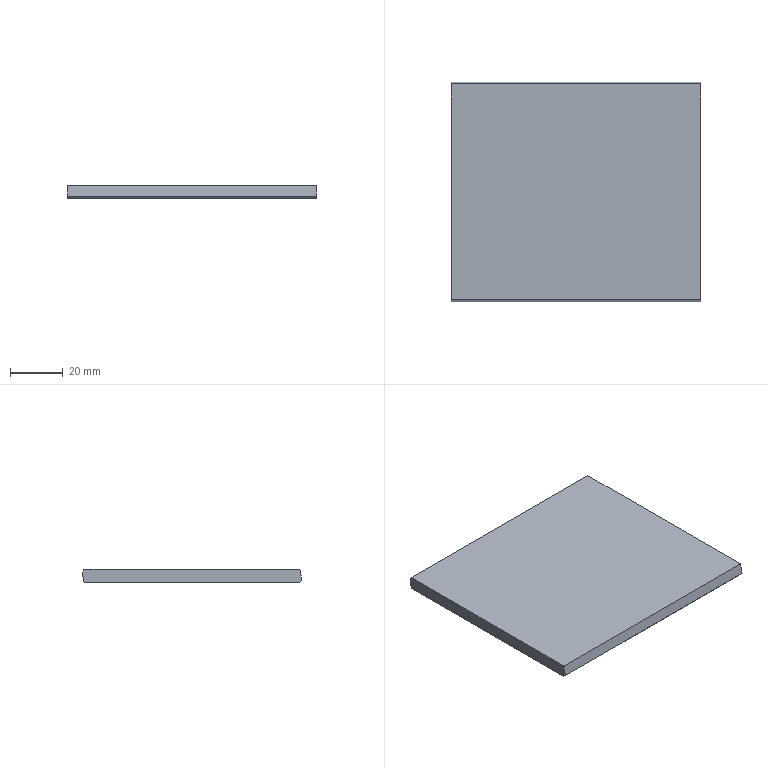Part | STEP file | Vibrator side plate_default | 1 solid | 8 faces | box 95 x 83.558 x 5 mm | volume 39344 mm3 | plane 8
STEP:
#1=CARTESIAN_POINT('',(0.,0.,0.));
#2=DIRECTION('',(0.,0.,1.));
#3=DIRECTION('',(1.,0.,0.));
#4=AXIS2_PLACEMENT_3D('',#1,#2,#3);
#5=CARTESIAN_POINT('',(-47.5,41.5,0.));
#6=VERTEX_POINT('',#5);
#7=CARTESIAN_POINT('',(-47.5,-40.5,0.));
#8=VERTEX_POINT('',#7);
#9=CARTESIAN_POINT('',(-47.5,-41.5,0.));
#10=DIRECTION('',(0.,-1.,0.));
#11=VECTOR('',#10,1.);
#12=LINE('',#9,#11);
#13=CARTESIAN_POINT('',(-47.5,-40.618,5.));
#14=DIRECTION('',(1.,0.,0.));
#15=DIRECTION('',(0.,0.,-1.));
#16=AXIS2_PLACEMENT_3D('',#13,#14,#15);
#17=PLANE('',#16);
#18=CARTESIAN_POINT('',(5.,-0.8816));
#19=DIRECTION('',(0.,-1.));
#20=VECTOR('',#19,1.);
#21=LINE('',#18,#20);
#22=(GEOMETRIC_REPRESENTATION_CONTEXT(2)PARAMETRIC_REPRESENTATION_CONTEXT()REPRESENTATION_CONTEXT('',''));
#23=DEFINITIONAL_REPRESENTATION('',(#21),#22);
#24=PCURVE('',#17,#23);
#25=CARTESIAN_POINT('',(0.,0.,0.));
#26=DIRECTION('',(0.,0.,1.));
#27=DIRECTION('',(1.,0.,0.));
#28=AXIS2_PLACEMENT_3D('',#25,#26,#27);
#29=PLANE('',#28);
#30=CARTESIAN_POINT('',(-47.5,-41.5));
#31=DIRECTION('',(0.,-1.));
#32=VECTOR('',#31,1.);
#33=LINE('',#30,#32);
#34=(GEOMETRIC_REPRESENTATION_CONTEXT(2)PARAMETRIC_REPRESENTATION_CONTEXT()REPRESENTATION_CONTEXT('',''));
#35=DEFINITIONAL_REPRESENTATION('',(#33),#34);
#36=PCURVE('',#29,#35);
#37=SURFACE_CURVE('',#12,(#24,#36),.PCURVE_S1.);
#38=EDGE_CURVE('',#6,#8,#37,.T.);
#39=ORIENTED_EDGE('',*,*,#38,.T.);
#40=CARTESIAN_POINT('',(-47.5,-41.35,0.8501));
#41=VERTEX_POINT('',#40);
#42=CARTESIAN_POINT('',(-47.5,-41.35,0.8501));
#43=DIRECTION('',(0.,-0.7071,0.7071));
#44=VECTOR('',#43,1.);
#45=LINE('',#42,#44);
#46=CARTESIAN_POINT('',(4.15,-0.7317));
#47=DIRECTION('',(-0.7071,-0.7071));
#48=VECTOR('',#47,1.);
#49=LINE('',#46,#48);
#50=(GEOMETRIC_REPRESENTATION_CONTEXT(2)PARAMETRIC_REPRESENTATION_CONTEXT()REPRESENTATION_CONTEXT('',''));
#51=DEFINITIONAL_REPRESENTATION('',(#49),#50);
#52=PCURVE('',#17,#51);
#53=CARTESIAN_POINT('',(47.5,-41.35,0.8501));
#54=DIRECTION('',(0.,0.7071,0.7071));
#55=DIRECTION('',(1.,0.,0.));
#56=AXIS2_PLACEMENT_3D('',#53,#54,#55);
#57=PLANE('',#56);
#58=CARTESIAN_POINT('',(-95.,0.));
#59=DIRECTION('',(0.,-1.));
#60=VECTOR('',#59,1.);
#61=LINE('',#58,#60);
#62=(GEOMETRIC_REPRESENTATION_CONTEXT(2)PARAMETRIC_REPRESENTATION_CONTEXT()REPRESENTATION_CONTEXT('',''));
#63=DEFINITIONAL_REPRESENTATION('',(#61),#62);
#64=PCURVE('',#57,#63);
#65=SURFACE_CURVE('',#45,(#52,#64),.PCURVE_S1.);
#66=EDGE_CURVE('',#8,#41,#65,.T.);
#67=ORIENTED_EDGE('',*,*,#66,.T.);
#68=CARTESIAN_POINT('',(-47.5,-40.618,5.));
#69=VERTEX_POINT('',#68);
#70=CARTESIAN_POINT('',(-47.5,-40.618,5.));
#71=DIRECTION('',(0.,-0.1736,-0.9848));
#72=VECTOR('',#71,1.);
#73=LINE('',#70,#72);
#74=CARTESIAN_POINT('',(0.,0.));
#75=DIRECTION('',(0.9848,-0.1736));
#76=VECTOR('',#75,1.);
#77=LINE('',#74,#76);
#78=(GEOMETRIC_REPRESENTATION_CONTEXT(2)PARAMETRIC_REPRESENTATION_CONTEXT()REPRESENTATION_CONTEXT('',''));
#79=DEFINITIONAL_REPRESENTATION('',(#77),#78);
#80=PCURVE('',#17,#79);
#81=CARTESIAN_POINT('',(47.5,-40.618,5.));
#82=DIRECTION('',(0.,0.9848,-0.1736));
#83=DIRECTION('',(0.,0.1736,0.9848));
#84=AXIS2_PLACEMENT_3D('',#81,#82,#83);
#85=PLANE('',#84);
#86=CARTESIAN_POINT('',(0.,-95.));
#87=DIRECTION('',(-1.,0.));
#88=VECTOR('',#87,1.);
#89=LINE('',#86,#88);
#90=(GEOMETRIC_REPRESENTATION_CONTEXT(2)PARAMETRIC_REPRESENTATION_CONTEXT()REPRESENTATION_CONTEXT('',''));
#91=DEFINITIONAL_REPRESENTATION('',(#89),#90);
#92=PCURVE('',#85,#91);
#93=SURFACE_CURVE('',#73,(#80,#92),.PCURVE_S1.);
#94=EDGE_CURVE('',#69,#41,#93,.T.);
#95=ORIENTED_EDGE('',*,*,#94,.F.);
#96=CARTESIAN_POINT('',(-47.5,41.518,5.));
#97=VERTEX_POINT('',#96);
#98=CARTESIAN_POINT('',(-47.5,-40.618,5.));
#99=DIRECTION('',(0.,-1.,0.));
#100=VECTOR('',#99,1.);
#101=LINE('',#98,#100);
#102=CARTESIAN_POINT('',(0.,0.));
#103=DIRECTION('',(0.,-1.));
#104=VECTOR('',#103,1.);
#105=LINE('',#102,#104);
#106=(GEOMETRIC_REPRESENTATION_CONTEXT(2)PARAMETRIC_REPRESENTATION_CONTEXT()REPRESENTATION_CONTEXT('',''));
#107=DEFINITIONAL_REPRESENTATION('',(#105),#106);
#108=PCURVE('',#17,#107);
#109=CARTESIAN_POINT('',(0.,0.8816,5.));
#110=DIRECTION('',(0.,0.,1.));
#111=DIRECTION('',(1.,0.,0.));
#112=AXIS2_PLACEMENT_3D('',#109,#110,#111);
#113=PLANE('',#112);
#114=CARTESIAN_POINT('',(-47.5,-41.5));
#115=DIRECTION('',(0.,-1.));
#116=VECTOR('',#115,1.);
#117=LINE('',#114,#116);
#118=(GEOMETRIC_REPRESENTATION_CONTEXT(2)PARAMETRIC_REPRESENTATION_CONTEXT()REPRESENTATION_CONTEXT('',''));
#119=DEFINITIONAL_REPRESENTATION('',(#117),#118);
#120=PCURVE('',#113,#119);
#121=SURFACE_CURVE('',#101,(#108,#120),.PCURVE_S1.);
#122=EDGE_CURVE('',#97,#69,#121,.T.);
#123=ORIENTED_EDGE('',*,*,#122,.F.);
#124=CARTESIAN_POINT('',(-47.5,42.208,4.015));
#125=VERTEX_POINT('',#124);
#126=CARTESIAN_POINT('',(-47.5,41.518,5.));
#127=DIRECTION('',(0.,0.5736,-0.8192));
#128=VECTOR('',#127,1.);
#129=LINE('',#126,#128);
#130=CARTESIAN_POINT('',(0.,82.137));
#131=DIRECTION('',(0.8192,0.5736));
#132=VECTOR('',#131,1.);
#133=LINE('',#130,#132);
#134=(GEOMETRIC_REPRESENTATION_CONTEXT(2)PARAMETRIC_REPRESENTATION_CONTEXT()REPRESENTATION_CONTEXT('',''));
#135=DEFINITIONAL_REPRESENTATION('',(#133),#134);
#136=PCURVE('',#17,#135);
#137=CARTESIAN_POINT('',(0.,41.518,5.));
#138=DIRECTION('',(0.,0.8192,0.5736));
#139=DIRECTION('',(1.,0.,0.));
#140=AXIS2_PLACEMENT_3D('',#137,#138,#139);
#141=PLANE('',#140);
#142=CARTESIAN_POINT('',(-47.5,0.));
#143=DIRECTION('',(0.,1.));
#144=VECTOR('',#143,1.);
#145=LINE('',#142,#144);
#146=(GEOMETRIC_REPRESENTATION_CONTEXT(2)PARAMETRIC_REPRESENTATION_CONTEXT()REPRESENTATION_CONTEXT('',''));
#147=DEFINITIONAL_REPRESENTATION('',(#145),#146);
#148=PCURVE('',#141,#147);
#149=SURFACE_CURVE('',#129,(#136,#148),.PCURVE_S1.);
#150=EDGE_CURVE('',#97,#125,#149,.T.);
#151=ORIENTED_EDGE('',*,*,#150,.T.);
#152=CARTESIAN_POINT('',(-47.5,42.382,5.));
#153=DIRECTION('',(0.,-0.1736,-0.9848));
#154=VECTOR('',#153,1.);
#155=LINE('',#152,#154);
#156=CARTESIAN_POINT('',(0.,83.));
#157=DIRECTION('',(0.9848,-0.1736));
#158=VECTOR('',#157,1.);
#159=LINE('',#156,#158);
#160=(GEOMETRIC_REPRESENTATION_CONTEXT(2)PARAMETRIC_REPRESENTATION_CONTEXT()REPRESENTATION_CONTEXT('',''));
#161=DEFINITIONAL_REPRESENTATION('',(#159),#160);
#162=PCURVE('',#17,#161);
#163=CARTESIAN_POINT('',(47.5,42.382,5.));
#164=DIRECTION('',(0.,-0.9848,0.1736));
#165=DIRECTION('',(0.,-0.1736,-0.9848));
#166=AXIS2_PLACEMENT_3D('',#163,#164,#165);
#167=PLANE('',#166);
#168=CARTESIAN_POINT('',(0.,-95.));
#169=DIRECTION('',(1.,0.));
#170=VECTOR('',#169,1.);
#171=LINE('',#168,#170);
#172=(GEOMETRIC_REPRESENTATION_CONTEXT(2)PARAMETRIC_REPRESENTATION_CONTEXT()REPRESENTATION_CONTEXT('',''));
#173=DEFINITIONAL_REPRESENTATION('',(#171),#172);
#174=PCURVE('',#167,#173);
#175=SURFACE_CURVE('',#155,(#162,#174),.PCURVE_S1.);
#176=EDGE_CURVE('',#125,#6,#175,.T.);
#177=ORIENTED_EDGE('',*,*,#176,.T.);
#178=EDGE_LOOP('',(#39,#67,#95,#123,#151,#177));
#179=FACE_BOUND('',#178,.T.);
#180=ADVANCED_FACE('',(#179),#17,.F.);
#181=ORIENTED_EDGE('',*,*,#94,.T.);
#182=CARTESIAN_POINT('',(47.5,-41.35,0.8501));
#183=VERTEX_POINT('',#182);
#184=CARTESIAN_POINT('',(47.5,-41.35,0.8501));
#185=DIRECTION('',(1.,0.,0.));
#186=VECTOR('',#185,1.);
#187=LINE('',#184,#186);
#188=CARTESIAN_POINT('',(-4.214,0.));
#189=DIRECTION('',(0.,1.));
#190=VECTOR('',#189,1.);
#191=LINE('',#188,#190);
#192=(GEOMETRIC_REPRESENTATION_CONTEXT(2)PARAMETRIC_REPRESENTATION_CONTEXT()REPRESENTATION_CONTEXT('',''));
#193=DEFINITIONAL_REPRESENTATION('',(#191),#192);
#194=PCURVE('',#85,#193);
#195=CARTESIAN_POINT('',(0.,0.));
#196=DIRECTION('',(1.,0.));
#197=VECTOR('',#196,1.);
#198=LINE('',#195,#197);
#199=(GEOMETRIC_REPRESENTATION_CONTEXT(2)PARAMETRIC_REPRESENTATION_CONTEXT()REPRESENTATION_CONTEXT('',''));
#200=DEFINITIONAL_REPRESENTATION('',(#198),#199);
#201=PCURVE('',#57,#200);
#202=SURFACE_CURVE('',#187,(#194,#201),.PCURVE_S1.);
#203=EDGE_CURVE('',#41,#183,#202,.T.);
#204=ORIENTED_EDGE('',*,*,#203,.T.);
#205=CARTESIAN_POINT('',(47.5,-40.618,5.));
#206=VERTEX_POINT('',#205);
#207=CARTESIAN_POINT('',(47.5,-40.618,5.));
#208=DIRECTION('',(0.,-0.1736,-0.9848));
#209=VECTOR('',#208,1.);
#210=LINE('',#207,#209);
#211=CARTESIAN_POINT('',(0.,0.));
#212=DIRECTION('',(-1.,0.));
#213=VECTOR('',#212,1.);
#214=LINE('',#211,#213);
#215=(GEOMETRIC_REPRESENTATION_CONTEXT(2)PARAMETRIC_REPRESENTATION_CONTEXT()REPRESENTATION_CONTEXT('',''));
#216=DEFINITIONAL_REPRESENTATION('',(#214),#215);
#217=PCURVE('',#85,#216);
#218=CARTESIAN_POINT('',(47.5,-40.618,5.));
#219=DIRECTION('',(-1.,0.,0.));
#220=DIRECTION('',(0.,0.,1.));
#221=AXIS2_PLACEMENT_3D('',#218,#219,#220);
#222=PLANE('',#221);
#223=CARTESIAN_POINT('',(0.,0.));
#224=DIRECTION('',(-0.9848,-0.1736));
#225=VECTOR('',#224,1.);
#226=LINE('',#223,#225);
#227=(GEOMETRIC_REPRESENTATION_CONTEXT(2)PARAMETRIC_REPRESENTATION_CONTEXT()REPRESENTATION_CONTEXT('',''));
#228=DEFINITIONAL_REPRESENTATION('',(#226),#227);
#229=PCURVE('',#222,#228);
#230=SURFACE_CURVE('',#210,(#217,#229),.PCURVE_S1.);
#231=EDGE_CURVE('',#206,#183,#230,.T.);
#232=ORIENTED_EDGE('',*,*,#231,.F.);
#233=CARTESIAN_POINT('',(47.5,-40.618,5.));
#234=DIRECTION('',(1.,0.,0.));
#235=VECTOR('',#234,1.);
#236=LINE('',#233,#235);
#237=CARTESIAN_POINT('',(0.,0.));
#238=DIRECTION('',(0.,1.));
#239=VECTOR('',#238,1.);
#240=LINE('',#237,#239);
#241=(GEOMETRIC_REPRESENTATION_CONTEXT(2)PARAMETRIC_REPRESENTATION_CONTEXT()REPRESENTATION_CONTEXT('',''));
#242=DEFINITIONAL_REPRESENTATION('',(#240),#241);
#243=PCURVE('',#85,#242);
#244=CARTESIAN_POINT('',(47.5,-41.5));
#245=DIRECTION('',(1.,0.));
#246=VECTOR('',#245,1.);
#247=LINE('',#244,#246);
#248=(GEOMETRIC_REPRESENTATION_CONTEXT(2)PARAMETRIC_REPRESENTATION_CONTEXT()REPRESENTATION_CONTEXT('',''));
#249=DEFINITIONAL_REPRESENTATION('',(#247),#248);
#250=PCURVE('',#113,#249);
#251=SURFACE_CURVE('',#236,(#243,#250),.PCURVE_S1.);
#252=EDGE_CURVE('',#69,#206,#251,.T.);
#253=ORIENTED_EDGE('',*,*,#252,.F.);
#254=EDGE_LOOP('',(#181,#204,#232,#253));
#255=FACE_BOUND('',#254,.T.);
#256=ADVANCED_FACE('',(#255),#85,.F.);
#257=ORIENTED_EDGE('',*,*,#231,.T.);
#258=CARTESIAN_POINT('',(47.5,-40.5,0.));
#259=VERTEX_POINT('',#258);
#260=CARTESIAN_POINT('',(47.5,-41.35,0.8501));
#261=DIRECTION('',(0.,0.7071,-0.7071));
#262=VECTOR('',#261,1.);
#263=LINE('',#260,#262);
#264=CARTESIAN_POINT('',(-4.15,-0.7317));
#265=DIRECTION('',(-0.7071,0.7071));
#266=VECTOR('',#265,1.);
#267=LINE('',#264,#266);
#268=(GEOMETRIC_REPRESENTATION_CONTEXT(2)PARAMETRIC_REPRESENTATION_CONTEXT()REPRESENTATION_CONTEXT('',''));
#269=DEFINITIONAL_REPRESENTATION('',(#267),#268);
#270=PCURVE('',#222,#269);
#271=CARTESIAN_POINT('',(0.,0.));
#272=DIRECTION('',(0.,1.));
#273=VECTOR('',#272,1.);
#274=LINE('',#271,#273);
#275=(GEOMETRIC_REPRESENTATION_CONTEXT(2)PARAMETRIC_REPRESENTATION_CONTEXT()REPRESENTATION_CONTEXT('',''));
#276=DEFINITIONAL_REPRESENTATION('',(#274),#275);
#277=PCURVE('',#57,#276);
#278=SURFACE_CURVE('',#263,(#270,#277),.PCURVE_S1.);
#279=EDGE_CURVE('',#183,#259,#278,.T.);
#280=ORIENTED_EDGE('',*,*,#279,.T.);
#281=CARTESIAN_POINT('',(47.5,41.5,0.));
#282=VERTEX_POINT('',#281);
#283=CARTESIAN_POINT('',(47.5,-41.5,0.));
#284=DIRECTION('',(0.,1.,0.));
#285=VECTOR('',#284,1.);
#286=LINE('',#283,#285);
#287=CARTESIAN_POINT('',(-5.,-0.8816));
#288=DIRECTION('',(0.,1.));
#289=VECTOR('',#288,1.);
#290=LINE('',#287,#289);
#291=(GEOMETRIC_REPRESENTATION_CONTEXT(2)PARAMETRIC_REPRESENTATION_CONTEXT()REPRESENTATION_CONTEXT('',''));
#292=DEFINITIONAL_REPRESENTATION('',(#290),#291);
#293=PCURVE('',#222,#292);
#294=CARTESIAN_POINT('',(47.5,-41.5));
#295=DIRECTION('',(0.,1.));
#296=VECTOR('',#295,1.);
#297=LINE('',#294,#296);
#298=(GEOMETRIC_REPRESENTATION_CONTEXT(2)PARAMETRIC_REPRESENTATION_CONTEXT()REPRESENTATION_CONTEXT('',''));
#299=DEFINITIONAL_REPRESENTATION('',(#297),#298);
#300=PCURVE('',#29,#299);
#301=SURFACE_CURVE('',#286,(#293,#300),.PCURVE_S1.);
#302=EDGE_CURVE('',#259,#282,#301,.T.);
#303=ORIENTED_EDGE('',*,*,#302,.T.);
#304=CARTESIAN_POINT('',(47.5,42.208,4.015));
#305=VERTEX_POINT('',#304);
#306=CARTESIAN_POINT('',(47.5,42.382,5.));
#307=DIRECTION('',(0.,-0.1736,-0.9848));
#308=VECTOR('',#307,1.);
#309=LINE('',#306,#308);
#310=CARTESIAN_POINT('',(0.,83.));
#311=DIRECTION('',(-0.9848,-0.1736));
#312=VECTOR('',#311,1.);
#313=LINE('',#310,#312);
#314=(GEOMETRIC_REPRESENTATION_CONTEXT(2)PARAMETRIC_REPRESENTATION_CONTEXT()REPRESENTATION_CONTEXT('',''));
#315=DEFINITIONAL_REPRESENTATION('',(#313),#314);
#316=PCURVE('',#222,#315);
#317=CARTESIAN_POINT('',(0.,0.));
#318=DIRECTION('',(1.,0.));
#319=VECTOR('',#318,1.);
#320=LINE('',#317,#319);
#321=(GEOMETRIC_REPRESENTATION_CONTEXT(2)PARAMETRIC_REPRESENTATION_CONTEXT()REPRESENTATION_CONTEXT('',''));
#322=DEFINITIONAL_REPRESENTATION('',(#320),#321);
#323=PCURVE('',#167,#322);
#324=SURFACE_CURVE('',#309,(#316,#323),.PCURVE_S1.);
#325=EDGE_CURVE('',#305,#282,#324,.T.);
#326=ORIENTED_EDGE('',*,*,#325,.F.);
#327=CARTESIAN_POINT('',(47.5,41.518,5.));
#328=VERTEX_POINT('',#327);
#329=CARTESIAN_POINT('',(47.5,41.518,5.));
#330=DIRECTION('',(0.,-0.5736,0.8192));
#331=VECTOR('',#330,1.);
#332=LINE('',#329,#331);
#333=CARTESIAN_POINT('',(0.,82.137));
#334=DIRECTION('',(0.8192,-0.5736));
#335=VECTOR('',#334,1.);
#336=LINE('',#333,#335);
#337=(GEOMETRIC_REPRESENTATION_CONTEXT(2)PARAMETRIC_REPRESENTATION_CONTEXT()REPRESENTATION_CONTEXT('',''));
#338=DEFINITIONAL_REPRESENTATION('',(#336),#337);
#339=PCURVE('',#222,#338);
#340=CARTESIAN_POINT('',(47.5,0.));
#341=DIRECTION('',(0.,-1.));
#342=VECTOR('',#341,1.);
#343=LINE('',#340,#342);
#344=(GEOMETRIC_REPRESENTATION_CONTEXT(2)PARAMETRIC_REPRESENTATION_CONTEXT()REPRESENTATION_CONTEXT('',''));
#345=DEFINITIONAL_REPRESENTATION('',(#343),#344);
#346=PCURVE('',#141,#345);
#347=SURFACE_CURVE('',#332,(#339,#346),.PCURVE_S1.);
#348=EDGE_CURVE('',#305,#328,#347,.T.);
#349=ORIENTED_EDGE('',*,*,#348,.T.);
#350=CARTESIAN_POINT('',(47.5,-40.618,5.));
#351=DIRECTION('',(0.,1.,0.));
#352=VECTOR('',#351,1.);
#353=LINE('',#350,#352);
#354=CARTESIAN_POINT('',(0.,0.));
#355=DIRECTION('',(0.,1.));
#356=VECTOR('',#355,1.);
#357=LINE('',#354,#356);
#358=(GEOMETRIC_REPRESENTATION_CONTEXT(2)PARAMETRIC_REPRESENTATION_CONTEXT()REPRESENTATION_CONTEXT('',''));
#359=DEFINITIONAL_REPRESENTATION('',(#357),#358);
#360=PCURVE('',#222,#359);
#361=CARTESIAN_POINT('',(47.5,-41.5));
#362=DIRECTION('',(0.,1.));
#363=VECTOR('',#362,1.);
#364=LINE('',#361,#363);
#365=(GEOMETRIC_REPRESENTATION_CONTEXT(2)PARAMETRIC_REPRESENTATION_CONTEXT()REPRESENTATION_CONTEXT('',''));
#366=DEFINITIONAL_REPRESENTATION('',(#364),#365);
#367=PCURVE('',#113,#366);
#368=SURFACE_CURVE('',#353,(#360,#367),.PCURVE_S1.);
#369=EDGE_CURVE('',#206,#328,#368,.T.);
#370=ORIENTED_EDGE('',*,*,#369,.F.);
#371=EDGE_LOOP('',(#257,#280,#303,#326,#349,#370));
#372=FACE_BOUND('',#371,.T.);
#373=ADVANCED_FACE('',(#372),#222,.F.);
#374=ORIENTED_EDGE('',*,*,#176,.F.);
#375=CARTESIAN_POINT('',(47.5,42.208,4.015));
#376=DIRECTION('',(1.,0.,0.));
#377=VECTOR('',#376,1.);
#378=LINE('',#375,#377);
#379=CARTESIAN_POINT('',(1.,0.));
#380=DIRECTION('',(0.,1.));
#381=VECTOR('',#380,1.);
#382=LINE('',#379,#381);
#383=(GEOMETRIC_REPRESENTATION_CONTEXT(2)PARAMETRIC_REPRESENTATION_CONTEXT()REPRESENTATION_CONTEXT('',''));
#384=DEFINITIONAL_REPRESENTATION('',(#382),#383);
#385=PCURVE('',#167,#384);
#386=CARTESIAN_POINT('',(47.5,1.202));
#387=DIRECTION('',(1.,0.));
#388=VECTOR('',#387,1.);
#389=LINE('',#386,#388);
#390=(GEOMETRIC_REPRESENTATION_CONTEXT(2)PARAMETRIC_REPRESENTATION_CONTEXT()REPRESENTATION_CONTEXT('',''));
#391=DEFINITIONAL_REPRESENTATION('',(#389),#390);
#392=PCURVE('',#141,#391);
#393=SURFACE_CURVE('',#378,(#385,#392),.PCURVE_S1.);
#394=EDGE_CURVE('',#125,#305,#393,.T.);
#395=ORIENTED_EDGE('',*,*,#394,.T.);
#396=ORIENTED_EDGE('',*,*,#325,.T.);
#397=CARTESIAN_POINT('',(47.5,41.5,0.));
#398=DIRECTION('',(-1.,0.,0.));
#399=VECTOR('',#398,1.);
#400=LINE('',#397,#399);
#401=CARTESIAN_POINT('',(5.077,0.));
#402=DIRECTION('',(0.,-1.));
#403=VECTOR('',#402,1.);
#404=LINE('',#401,#403);
#405=(GEOMETRIC_REPRESENTATION_CONTEXT(2)PARAMETRIC_REPRESENTATION_CONTEXT()REPRESENTATION_CONTEXT('',''));
#406=DEFINITIONAL_REPRESENTATION('',(#404),#405);
#407=PCURVE('',#167,#406);
#408=CARTESIAN_POINT('',(47.5,41.5));
#409=DIRECTION('',(-1.,0.));
#410=VECTOR('',#409,1.);
#411=LINE('',#408,#410);
#412=(GEOMETRIC_REPRESENTATION_CONTEXT(2)PARAMETRIC_REPRESENTATION_CONTEXT()REPRESENTATION_CONTEXT('',''));
#413=DEFINITIONAL_REPRESENTATION('',(#411),#412);
#414=PCURVE('',#29,#413);
#415=SURFACE_CURVE('',#400,(#407,#414),.PCURVE_S1.);
#416=EDGE_CURVE('',#282,#6,#415,.T.);
#417=ORIENTED_EDGE('',*,*,#416,.T.);
#418=EDGE_LOOP('',(#374,#395,#396,#417));
#419=FACE_BOUND('',#418,.T.);
#420=ADVANCED_FACE('',(#419),#167,.F.);
#421=ORIENTED_EDGE('',*,*,#369,.T.);
#422=CARTESIAN_POINT('',(-47.5,41.518,5.));
#423=DIRECTION('',(-1.,0.,0.));
#424=VECTOR('',#423,1.);
#425=LINE('',#422,#424);
#426=CARTESIAN_POINT('',(-47.5,40.637));
#427=DIRECTION('',(-1.,0.));
#428=VECTOR('',#427,1.);
#429=LINE('',#426,#428);
#430=(GEOMETRIC_REPRESENTATION_CONTEXT(2)PARAMETRIC_REPRESENTATION_CONTEXT()REPRESENTATION_CONTEXT('',''));
#431=DEFINITIONAL_REPRESENTATION('',(#429),#430);
#432=PCURVE('',#113,#431);
#433=CARTESIAN_POINT('',(-47.5,0.));
#434=DIRECTION('',(-1.,0.));
#435=VECTOR('',#434,1.);
#436=LINE('',#433,#435);
#437=(GEOMETRIC_REPRESENTATION_CONTEXT(2)PARAMETRIC_REPRESENTATION_CONTEXT()REPRESENTATION_CONTEXT('',''));
#438=DEFINITIONAL_REPRESENTATION('',(#436),#437);
#439=PCURVE('',#141,#438);
#440=SURFACE_CURVE('',#425,(#432,#439),.PCURVE_S1.);
#441=EDGE_CURVE('',#328,#97,#440,.T.);
#442=ORIENTED_EDGE('',*,*,#441,.T.);
#443=ORIENTED_EDGE('',*,*,#122,.T.);
#444=ORIENTED_EDGE('',*,*,#252,.T.);
#445=EDGE_LOOP('',(#421,#442,#443,#444));
#446=FACE_BOUND('',#445,.T.);
#447=ADVANCED_FACE('',(#446),#113,.T.);
#448=ORIENTED_EDGE('',*,*,#302,.F.);
#449=CARTESIAN_POINT('',(0.,-40.5,0.));
#450=DIRECTION('',(-1.,0.,0.));
#451=VECTOR('',#450,1.);
#452=LINE('',#449,#451);
#453=CARTESIAN_POINT('',(0.,-40.5));
#454=DIRECTION('',(-1.,0.));
#455=VECTOR('',#454,1.);
#456=LINE('',#453,#455);
#457=(GEOMETRIC_REPRESENTATION_CONTEXT(2)PARAMETRIC_REPRESENTATION_CONTEXT()REPRESENTATION_CONTEXT('',''));
#458=DEFINITIONAL_REPRESENTATION('',(#456),#457);
#459=PCURVE('',#29,#458);
#460=CARTESIAN_POINT('',(-47.5,1.202));
#461=DIRECTION('',(-1.,0.));
#462=VECTOR('',#461,1.);
#463=LINE('',#460,#462);
#464=(GEOMETRIC_REPRESENTATION_CONTEXT(2)PARAMETRIC_REPRESENTATION_CONTEXT()REPRESENTATION_CONTEXT('',''));
#465=DEFINITIONAL_REPRESENTATION('',(#463),#464);
#466=PCURVE('',#57,#465);
#467=SURFACE_CURVE('',#452,(#459,#466),.PCURVE_S1.);
#468=EDGE_CURVE('',#259,#8,#467,.T.);
#469=ORIENTED_EDGE('',*,*,#468,.T.);
#470=ORIENTED_EDGE('',*,*,#38,.F.);
#471=ORIENTED_EDGE('',*,*,#416,.F.);
#472=EDGE_LOOP('',(#448,#469,#470,#471));
#473=FACE_BOUND('',#472,.T.);
#474=ADVANCED_FACE('',(#473),#29,.F.);
#475=ORIENTED_EDGE('',*,*,#66,.F.);
#476=ORIENTED_EDGE('',*,*,#468,.F.);
#477=ORIENTED_EDGE('',*,*,#279,.F.);
#478=ORIENTED_EDGE('',*,*,#203,.F.);
#479=EDGE_LOOP('',(#475,#476,#477,#478));
#480=FACE_BOUND('',#479,.T.);
#481=ADVANCED_FACE('',(#480),#57,.F.);
#482=ORIENTED_EDGE('',*,*,#348,.F.);
#483=ORIENTED_EDGE('',*,*,#394,.F.);
#484=ORIENTED_EDGE('',*,*,#150,.F.);
#485=ORIENTED_EDGE('',*,*,#441,.F.);
#486=EDGE_LOOP('',(#482,#483,#484,#485));
#487=FACE_BOUND('',#486,.T.);
#488=ADVANCED_FACE('',(#487),#141,.T.);
#489=CLOSED_SHELL('',(#180,#256,#373,#420,#447,#474,#481,#488));
#490=MANIFOLD_SOLID_BREP('',#489);
#491=(LENGTH_UNIT()NAMED_UNIT(*)SI_UNIT(.MILLI.,.METRE.));
#492=UNCERTAINTY_MEASURE_WITH_UNIT(LENGTH_MEASURE(0.0000001),#491,'','');
#493=(NAMED_UNIT(*)PLANE_ANGLE_UNIT()SI_UNIT($,.RADIAN.));
#494=(NAMED_UNIT(*)SI_UNIT($,.STERADIAN.)SOLID_ANGLE_UNIT());
#495=(GEOMETRIC_REPRESENTATION_CONTEXT(3)GLOBAL_UNCERTAINTY_ASSIGNED_CONTEXT((#492))GLOBAL_UNIT_ASSIGNED_CONTEXT((#491,#493,#494))REPRESENTATION_CONTEXT('',''));
#496=ADVANCED_BREP_SHAPE_REPRESENTATION('',(#4,#490),#495);